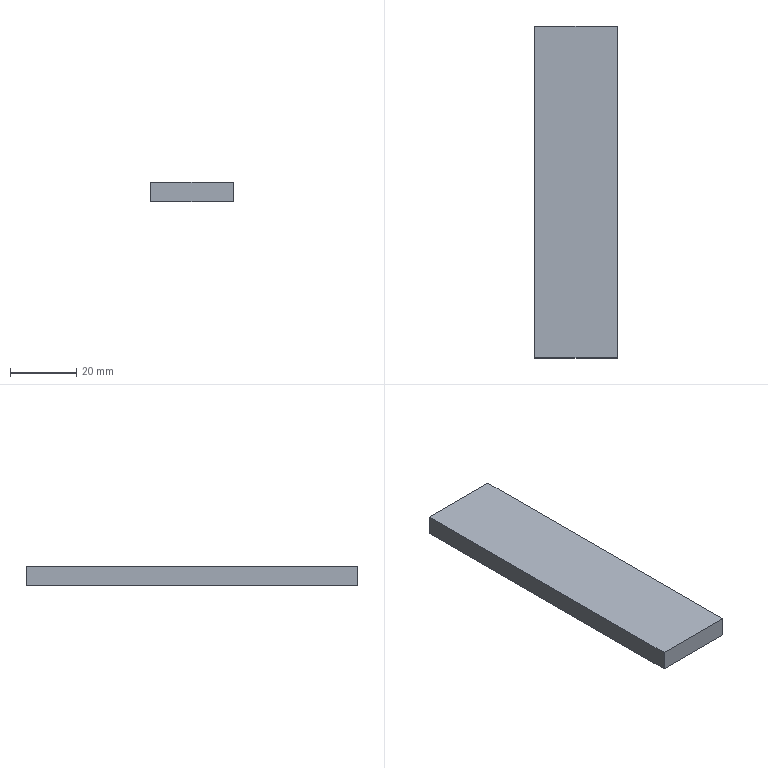Part | STEP file | 10-Part 25x100x6 | 1 solid | 6 faces | box 25 x 100 x 6 mm | volume 15000 mm3 | plane 6
STEP:
#1=CARTESIAN_POINT('',(0.,0.,0.));
#2=DIRECTION('',(0.,0.,1.));
#3=DIRECTION('',(1.,0.,0.));
#4=AXIS2_PLACEMENT_3D('',#1,#2,#3);
#5=CARTESIAN_POINT('',(0.,0.,0.));
#6=VERTEX_POINT('',#5);
#7=CARTESIAN_POINT('',(0.,-100.,0.));
#8=VERTEX_POINT('',#7);
#9=CARTESIAN_POINT('',(0.,0.,0.));
#10=DIRECTION('',(0.,-1.,0.));
#11=VECTOR('',#10,1.);
#12=LINE('',#9,#11);
#13=CARTESIAN_POINT('',(0.,0.,6.));
#14=DIRECTION('',(1.,0.,0.));
#15=DIRECTION('',(0.,1.,0.));
#16=AXIS2_PLACEMENT_3D('',#13,#14,#15);
#17=PLANE('',#16);
#18=CARTESIAN_POINT('',(0.,-6.));
#19=DIRECTION('',(-1.,0.));
#20=VECTOR('',#19,1.);
#21=LINE('',#18,#20);
#22=(GEOMETRIC_REPRESENTATION_CONTEXT(2)PARAMETRIC_REPRESENTATION_CONTEXT()REPRESENTATION_CONTEXT('',''));
#23=DEFINITIONAL_REPRESENTATION('',(#21),#22);
#24=PCURVE('',#17,#23);
#25=CARTESIAN_POINT('',(0.,0.,0.));
#26=DIRECTION('',(0.,0.,1.));
#27=DIRECTION('',(1.,0.,0.));
#28=AXIS2_PLACEMENT_3D('',#25,#26,#27);
#29=PLANE('',#28);
#30=CARTESIAN_POINT('',(0.,0.));
#31=DIRECTION('',(0.,-1.));
#32=VECTOR('',#31,1.);
#33=LINE('',#30,#32);
#34=(GEOMETRIC_REPRESENTATION_CONTEXT(2)PARAMETRIC_REPRESENTATION_CONTEXT()REPRESENTATION_CONTEXT('',''));
#35=DEFINITIONAL_REPRESENTATION('',(#33),#34);
#36=PCURVE('',#29,#35);
#37=SURFACE_CURVE('',#12,(#24,#36),.PCURVE_S1.);
#38=EDGE_CURVE('',#6,#8,#37,.T.);
#39=ORIENTED_EDGE('',*,*,#38,.T.);
#40=CARTESIAN_POINT('',(0.,-100.,6.));
#41=VERTEX_POINT('',#40);
#42=CARTESIAN_POINT('',(0.,-100.,6.));
#43=DIRECTION('',(0.,0.,-1.));
#44=VECTOR('',#43,1.);
#45=LINE('',#42,#44);
#46=CARTESIAN_POINT('',(-100.,0.));
#47=DIRECTION('',(0.,-1.));
#48=VECTOR('',#47,1.);
#49=LINE('',#46,#48);
#50=(GEOMETRIC_REPRESENTATION_CONTEXT(2)PARAMETRIC_REPRESENTATION_CONTEXT()REPRESENTATION_CONTEXT('',''));
#51=DEFINITIONAL_REPRESENTATION('',(#49),#50);
#52=PCURVE('',#17,#51);
#53=CARTESIAN_POINT('',(0.,-100.,6.));
#54=DIRECTION('',(0.,1.,0.));
#55=DIRECTION('',(0.,0.,1.));
#56=AXIS2_PLACEMENT_3D('',#53,#54,#55);
#57=PLANE('',#56);
#58=CARTESIAN_POINT('',(0.,0.));
#59=DIRECTION('',(-1.,0.));
#60=VECTOR('',#59,1.);
#61=LINE('',#58,#60);
#62=(GEOMETRIC_REPRESENTATION_CONTEXT(2)PARAMETRIC_REPRESENTATION_CONTEXT()REPRESENTATION_CONTEXT('',''));
#63=DEFINITIONAL_REPRESENTATION('',(#61),#62);
#64=PCURVE('',#57,#63);
#65=SURFACE_CURVE('',#45,(#52,#64),.PCURVE_S1.);
#66=EDGE_CURVE('',#41,#8,#65,.T.);
#67=ORIENTED_EDGE('',*,*,#66,.F.);
#68=CARTESIAN_POINT('',(0.,0.,6.));
#69=VERTEX_POINT('',#68);
#70=CARTESIAN_POINT('',(0.,0.,6.));
#71=DIRECTION('',(0.,-1.,0.));
#72=VECTOR('',#71,1.);
#73=LINE('',#70,#72);
#74=CARTESIAN_POINT('',(0.,0.));
#75=DIRECTION('',(-1.,0.));
#76=VECTOR('',#75,1.);
#77=LINE('',#74,#76);
#78=(GEOMETRIC_REPRESENTATION_CONTEXT(2)PARAMETRIC_REPRESENTATION_CONTEXT()REPRESENTATION_CONTEXT('',''));
#79=DEFINITIONAL_REPRESENTATION('',(#77),#78);
#80=PCURVE('',#17,#79);
#81=CARTESIAN_POINT('',(0.,0.,6.));
#82=DIRECTION('',(0.,0.,1.));
#83=DIRECTION('',(1.,0.,0.));
#84=AXIS2_PLACEMENT_3D('',#81,#82,#83);
#85=PLANE('',#84);
#86=CARTESIAN_POINT('',(0.,0.));
#87=DIRECTION('',(0.,-1.));
#88=VECTOR('',#87,1.);
#89=LINE('',#86,#88);
#90=(GEOMETRIC_REPRESENTATION_CONTEXT(2)PARAMETRIC_REPRESENTATION_CONTEXT()REPRESENTATION_CONTEXT('',''));
#91=DEFINITIONAL_REPRESENTATION('',(#89),#90);
#92=PCURVE('',#85,#91);
#93=SURFACE_CURVE('',#73,(#80,#92),.PCURVE_S1.);
#94=EDGE_CURVE('',#69,#41,#93,.T.);
#95=ORIENTED_EDGE('',*,*,#94,.F.);
#96=CARTESIAN_POINT('',(0.,0.,6.));
#97=DIRECTION('',(0.,0.,-1.));
#98=VECTOR('',#97,1.);
#99=LINE('',#96,#98);
#100=CARTESIAN_POINT('',(0.,0.));
#101=DIRECTION('',(0.,-1.));
#102=VECTOR('',#101,1.);
#103=LINE('',#100,#102);
#104=(GEOMETRIC_REPRESENTATION_CONTEXT(2)PARAMETRIC_REPRESENTATION_CONTEXT()REPRESENTATION_CONTEXT('',''));
#105=DEFINITIONAL_REPRESENTATION('',(#103),#104);
#106=PCURVE('',#17,#105);
#107=CARTESIAN_POINT('',(0.,0.,6.));
#108=DIRECTION('',(0.,-1.,0.));
#109=DIRECTION('',(0.,0.,-1.));
#110=AXIS2_PLACEMENT_3D('',#107,#108,#109);
#111=PLANE('',#110);
#112=CARTESIAN_POINT('',(0.,0.));
#113=DIRECTION('',(1.,0.));
#114=VECTOR('',#113,1.);
#115=LINE('',#112,#114);
#116=(GEOMETRIC_REPRESENTATION_CONTEXT(2)PARAMETRIC_REPRESENTATION_CONTEXT()REPRESENTATION_CONTEXT('',''));
#117=DEFINITIONAL_REPRESENTATION('',(#115),#116);
#118=PCURVE('',#111,#117);
#119=SURFACE_CURVE('',#99,(#106,#118),.PCURVE_S1.);
#120=EDGE_CURVE('',#69,#6,#119,.T.);
#121=ORIENTED_EDGE('',*,*,#120,.T.);
#122=EDGE_LOOP('',(#39,#67,#95,#121));
#123=FACE_BOUND('',#122,.T.);
#124=ADVANCED_FACE('',(#123),#17,.F.);
#125=CARTESIAN_POINT('',(25.,-100.,0.));
#126=VERTEX_POINT('',#125);
#127=CARTESIAN_POINT('',(0.,-100.,0.));
#128=DIRECTION('',(1.,0.,0.));
#129=VECTOR('',#128,1.);
#130=LINE('',#127,#129);
#131=CARTESIAN_POINT('',(-6.,0.));
#132=DIRECTION('',(0.,1.));
#133=VECTOR('',#132,1.);
#134=LINE('',#131,#133);
#135=(GEOMETRIC_REPRESENTATION_CONTEXT(2)PARAMETRIC_REPRESENTATION_CONTEXT()REPRESENTATION_CONTEXT('',''));
#136=DEFINITIONAL_REPRESENTATION('',(#134),#135);
#137=PCURVE('',#57,#136);
#138=CARTESIAN_POINT('',(0.,-100.));
#139=DIRECTION('',(1.,0.));
#140=VECTOR('',#139,1.);
#141=LINE('',#138,#140);
#142=(GEOMETRIC_REPRESENTATION_CONTEXT(2)PARAMETRIC_REPRESENTATION_CONTEXT()REPRESENTATION_CONTEXT('',''));
#143=DEFINITIONAL_REPRESENTATION('',(#141),#142);
#144=PCURVE('',#29,#143);
#145=SURFACE_CURVE('',#130,(#137,#144),.PCURVE_S1.);
#146=EDGE_CURVE('',#8,#126,#145,.T.);
#147=ORIENTED_EDGE('',*,*,#146,.T.);
#148=CARTESIAN_POINT('',(25.,-100.,6.));
#149=VERTEX_POINT('',#148);
#150=CARTESIAN_POINT('',(25.,-100.,6.));
#151=DIRECTION('',(0.,0.,-1.));
#152=VECTOR('',#151,1.);
#153=LINE('',#150,#152);
#154=CARTESIAN_POINT('',(0.,25.));
#155=DIRECTION('',(-1.,0.));
#156=VECTOR('',#155,1.);
#157=LINE('',#154,#156);
#158=(GEOMETRIC_REPRESENTATION_CONTEXT(2)PARAMETRIC_REPRESENTATION_CONTEXT()REPRESENTATION_CONTEXT('',''));
#159=DEFINITIONAL_REPRESENTATION('',(#157),#158);
#160=PCURVE('',#57,#159);
#161=CARTESIAN_POINT('',(25.,0.,6.));
#162=DIRECTION('',(-1.,0.,0.));
#163=DIRECTION('',(0.,-1.,0.));
#164=AXIS2_PLACEMENT_3D('',#161,#162,#163);
#165=PLANE('',#164);
#166=CARTESIAN_POINT('',(100.,0.));
#167=DIRECTION('',(0.,-1.));
#168=VECTOR('',#167,1.);
#169=LINE('',#166,#168);
#170=(GEOMETRIC_REPRESENTATION_CONTEXT(2)PARAMETRIC_REPRESENTATION_CONTEXT()REPRESENTATION_CONTEXT('',''));
#171=DEFINITIONAL_REPRESENTATION('',(#169),#170);
#172=PCURVE('',#165,#171);
#173=SURFACE_CURVE('',#153,(#160,#172),.PCURVE_S1.);
#174=EDGE_CURVE('',#149,#126,#173,.T.);
#175=ORIENTED_EDGE('',*,*,#174,.F.);
#176=CARTESIAN_POINT('',(0.,-100.,6.));
#177=DIRECTION('',(1.,0.,0.));
#178=VECTOR('',#177,1.);
#179=LINE('',#176,#178);
#180=CARTESIAN_POINT('',(0.,0.));
#181=DIRECTION('',(0.,1.));
#182=VECTOR('',#181,1.);
#183=LINE('',#180,#182);
#184=(GEOMETRIC_REPRESENTATION_CONTEXT(2)PARAMETRIC_REPRESENTATION_CONTEXT()REPRESENTATION_CONTEXT('',''));
#185=DEFINITIONAL_REPRESENTATION('',(#183),#184);
#186=PCURVE('',#57,#185);
#187=CARTESIAN_POINT('',(0.,-100.));
#188=DIRECTION('',(1.,0.));
#189=VECTOR('',#188,1.);
#190=LINE('',#187,#189);
#191=(GEOMETRIC_REPRESENTATION_CONTEXT(2)PARAMETRIC_REPRESENTATION_CONTEXT()REPRESENTATION_CONTEXT('',''));
#192=DEFINITIONAL_REPRESENTATION('',(#190),#191);
#193=PCURVE('',#85,#192);
#194=SURFACE_CURVE('',#179,(#186,#193),.PCURVE_S1.);
#195=EDGE_CURVE('',#41,#149,#194,.T.);
#196=ORIENTED_EDGE('',*,*,#195,.F.);
#197=ORIENTED_EDGE('',*,*,#66,.T.);
#198=EDGE_LOOP('',(#147,#175,#196,#197));
#199=FACE_BOUND('',#198,.T.);
#200=ADVANCED_FACE('',(#199),#57,.F.);
#201=CARTESIAN_POINT('',(25.,0.,0.));
#202=VERTEX_POINT('',#201);
#203=CARTESIAN_POINT('',(25.,0.,0.));
#204=DIRECTION('',(0.,1.,0.));
#205=VECTOR('',#204,1.);
#206=LINE('',#203,#205);
#207=CARTESIAN_POINT('',(0.,-6.));
#208=DIRECTION('',(-1.,0.));
#209=VECTOR('',#208,1.);
#210=LINE('',#207,#209);
#211=(GEOMETRIC_REPRESENTATION_CONTEXT(2)PARAMETRIC_REPRESENTATION_CONTEXT()REPRESENTATION_CONTEXT('',''));
#212=DEFINITIONAL_REPRESENTATION('',(#210),#211);
#213=PCURVE('',#165,#212);
#214=CARTESIAN_POINT('',(25.,0.));
#215=DIRECTION('',(0.,1.));
#216=VECTOR('',#215,1.);
#217=LINE('',#214,#216);
#218=(GEOMETRIC_REPRESENTATION_CONTEXT(2)PARAMETRIC_REPRESENTATION_CONTEXT()REPRESENTATION_CONTEXT('',''));
#219=DEFINITIONAL_REPRESENTATION('',(#217),#218);
#220=PCURVE('',#29,#219);
#221=SURFACE_CURVE('',#206,(#213,#220),.PCURVE_S1.);
#222=EDGE_CURVE('',#126,#202,#221,.T.);
#223=ORIENTED_EDGE('',*,*,#222,.T.);
#224=CARTESIAN_POINT('',(25.,0.,6.));
#225=VERTEX_POINT('',#224);
#226=CARTESIAN_POINT('',(25.,0.,6.));
#227=DIRECTION('',(0.,0.,-1.));
#228=VECTOR('',#227,1.);
#229=LINE('',#226,#228);
#230=CARTESIAN_POINT('',(0.,0.));
#231=DIRECTION('',(0.,-1.));
#232=VECTOR('',#231,1.);
#233=LINE('',#230,#232);
#234=(GEOMETRIC_REPRESENTATION_CONTEXT(2)PARAMETRIC_REPRESENTATION_CONTEXT()REPRESENTATION_CONTEXT('',''));
#235=DEFINITIONAL_REPRESENTATION('',(#233),#234);
#236=PCURVE('',#165,#235);
#237=CARTESIAN_POINT('',(0.,25.));
#238=DIRECTION('',(1.,0.));
#239=VECTOR('',#238,1.);
#240=LINE('',#237,#239);
#241=(GEOMETRIC_REPRESENTATION_CONTEXT(2)PARAMETRIC_REPRESENTATION_CONTEXT()REPRESENTATION_CONTEXT('',''));
#242=DEFINITIONAL_REPRESENTATION('',(#240),#241);
#243=PCURVE('',#111,#242);
#244=SURFACE_CURVE('',#229,(#236,#243),.PCURVE_S1.);
#245=EDGE_CURVE('',#225,#202,#244,.T.);
#246=ORIENTED_EDGE('',*,*,#245,.F.);
#247=CARTESIAN_POINT('',(25.,0.,6.));
#248=DIRECTION('',(0.,1.,0.));
#249=VECTOR('',#248,1.);
#250=LINE('',#247,#249);
#251=CARTESIAN_POINT('',(0.,0.));
#252=DIRECTION('',(-1.,0.));
#253=VECTOR('',#252,1.);
#254=LINE('',#251,#253);
#255=(GEOMETRIC_REPRESENTATION_CONTEXT(2)PARAMETRIC_REPRESENTATION_CONTEXT()REPRESENTATION_CONTEXT('',''));
#256=DEFINITIONAL_REPRESENTATION('',(#254),#255);
#257=PCURVE('',#165,#256);
#258=CARTESIAN_POINT('',(25.,0.));
#259=DIRECTION('',(0.,1.));
#260=VECTOR('',#259,1.);
#261=LINE('',#258,#260);
#262=(GEOMETRIC_REPRESENTATION_CONTEXT(2)PARAMETRIC_REPRESENTATION_CONTEXT()REPRESENTATION_CONTEXT('',''));
#263=DEFINITIONAL_REPRESENTATION('',(#261),#262);
#264=PCURVE('',#85,#263);
#265=SURFACE_CURVE('',#250,(#257,#264),.PCURVE_S1.);
#266=EDGE_CURVE('',#149,#225,#265,.T.);
#267=ORIENTED_EDGE('',*,*,#266,.F.);
#268=ORIENTED_EDGE('',*,*,#174,.T.);
#269=EDGE_LOOP('',(#223,#246,#267,#268));
#270=FACE_BOUND('',#269,.T.);
#271=ADVANCED_FACE('',(#270),#165,.F.);
#272=CARTESIAN_POINT('',(0.,0.,0.));
#273=DIRECTION('',(-1.,0.,0.));
#274=VECTOR('',#273,1.);
#275=LINE('',#272,#274);
#276=CARTESIAN_POINT('',(6.,0.));
#277=DIRECTION('',(0.,-1.));
#278=VECTOR('',#277,1.);
#279=LINE('',#276,#278);
#280=(GEOMETRIC_REPRESENTATION_CONTEXT(2)PARAMETRIC_REPRESENTATION_CONTEXT()REPRESENTATION_CONTEXT('',''));
#281=DEFINITIONAL_REPRESENTATION('',(#279),#280);
#282=PCURVE('',#111,#281);
#283=CARTESIAN_POINT('',(0.,0.));
#284=DIRECTION('',(-1.,0.));
#285=VECTOR('',#284,1.);
#286=LINE('',#283,#285);
#287=(GEOMETRIC_REPRESENTATION_CONTEXT(2)PARAMETRIC_REPRESENTATION_CONTEXT()REPRESENTATION_CONTEXT('',''));
#288=DEFINITIONAL_REPRESENTATION('',(#286),#287);
#289=PCURVE('',#29,#288);
#290=SURFACE_CURVE('',#275,(#282,#289),.PCURVE_S1.);
#291=EDGE_CURVE('',#202,#6,#290,.T.);
#292=ORIENTED_EDGE('',*,*,#291,.T.);
#293=ORIENTED_EDGE('',*,*,#120,.F.);
#294=CARTESIAN_POINT('',(0.,0.,6.));
#295=DIRECTION('',(-1.,0.,0.));
#296=VECTOR('',#295,1.);
#297=LINE('',#294,#296);
#298=CARTESIAN_POINT('',(0.,0.));
#299=DIRECTION('',(0.,-1.));
#300=VECTOR('',#299,1.);
#301=LINE('',#298,#300);
#302=(GEOMETRIC_REPRESENTATION_CONTEXT(2)PARAMETRIC_REPRESENTATION_CONTEXT()REPRESENTATION_CONTEXT('',''));
#303=DEFINITIONAL_REPRESENTATION('',(#301),#302);
#304=PCURVE('',#111,#303);
#305=CARTESIAN_POINT('',(0.,0.));
#306=DIRECTION('',(-1.,0.));
#307=VECTOR('',#306,1.);
#308=LINE('',#305,#307);
#309=(GEOMETRIC_REPRESENTATION_CONTEXT(2)PARAMETRIC_REPRESENTATION_CONTEXT()REPRESENTATION_CONTEXT('',''));
#310=DEFINITIONAL_REPRESENTATION('',(#308),#309);
#311=PCURVE('',#85,#310);
#312=SURFACE_CURVE('',#297,(#304,#311),.PCURVE_S1.);
#313=EDGE_CURVE('',#225,#69,#312,.T.);
#314=ORIENTED_EDGE('',*,*,#313,.F.);
#315=ORIENTED_EDGE('',*,*,#245,.T.);
#316=EDGE_LOOP('',(#292,#293,#314,#315));
#317=FACE_BOUND('',#316,.T.);
#318=ADVANCED_FACE('',(#317),#111,.F.);
#319=ORIENTED_EDGE('',*,*,#94,.T.);
#320=ORIENTED_EDGE('',*,*,#195,.T.);
#321=ORIENTED_EDGE('',*,*,#266,.T.);
#322=ORIENTED_EDGE('',*,*,#313,.T.);
#323=EDGE_LOOP('',(#319,#320,#321,#322));
#324=FACE_BOUND('',#323,.T.);
#325=ADVANCED_FACE('',(#324),#85,.T.);
#326=ORIENTED_EDGE('',*,*,#38,.F.);
#327=ORIENTED_EDGE('',*,*,#291,.F.);
#328=ORIENTED_EDGE('',*,*,#222,.F.);
#329=ORIENTED_EDGE('',*,*,#146,.F.);
#330=EDGE_LOOP('',(#326,#327,#328,#329));
#331=FACE_BOUND('',#330,.T.);
#332=ADVANCED_FACE('',(#331),#29,.F.);
#333=CLOSED_SHELL('',(#124,#200,#271,#318,#325,#332));
#334=MANIFOLD_SOLID_BREP('',#333);
#335=(LENGTH_UNIT()NAMED_UNIT(*)SI_UNIT(.MILLI.,.METRE.));
#336=UNCERTAINTY_MEASURE_WITH_UNIT(LENGTH_MEASURE(0.0000001),#335,'','');
#337=(NAMED_UNIT(*)PLANE_ANGLE_UNIT()SI_UNIT($,.RADIAN.));
#338=(NAMED_UNIT(*)SI_UNIT($,.STERADIAN.)SOLID_ANGLE_UNIT());
#339=(GEOMETRIC_REPRESENTATION_CONTEXT(3)GLOBAL_UNCERTAINTY_ASSIGNED_CONTEXT((#336))GLOBAL_UNIT_ASSIGNED_CONTEXT((#335,#337,#338))REPRESENTATION_CONTEXT('',''));
#340=ADVANCED_BREP_SHAPE_REPRESENTATION('',(#4,#334),#339);